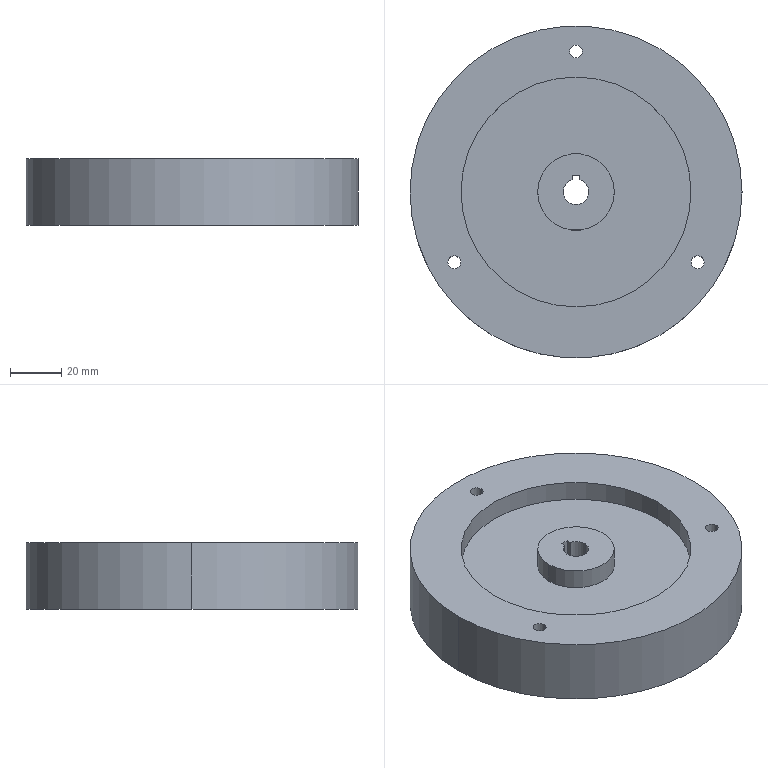Part | SolidWorks | features ICE 3, Extrusion 1 | 1 solid | 28 faces | box 130 x 130 x 26 mm | volume 250937 mm3 | cylinder 19 | plane 9 | commonest cylinder face diameters 5 x6 30 x4 90 x4 10 x3 130 x2
STEP:
#1=CARTESIAN_POINT('',(-15.,0.,8.));
#2=VERTEX_POINT('',#1);
#3=CARTESIAN_POINT('',(15.,0.,8.));
#4=VERTEX_POINT('',#3);
#5=CARTESIAN_POINT('',(0.,0.,8.));
#6=DIRECTION('',(0.,0.,-1.));
#7=DIRECTION('',(-1.,0.,0.));
#8=AXIS2_PLACEMENT_3D('',#5,#6,#7);
#9=CIRCLE('',#8,15.);
#10=EDGE_CURVE('',#2,#4,#9,.T.);
#11=ORIENTED_EDGE('',*,*,#10,.T.);
#12=CARTESIAN_POINT('',(15.,0.,0.));
#13=VERTEX_POINT('',#12);
#14=CARTESIAN_POINT('',(15.,0.,8.));
#15=DIRECTION('',(0.,0.,-1.));
#16=VECTOR('',#15,1000.);
#17=LINE('',#14,#16);
#18=EDGE_CURVE('',#4,#13,#17,.T.);
#19=ORIENTED_EDGE('',*,*,#18,.T.);
#20=CARTESIAN_POINT('',(-15.,0.,0.));
#21=VERTEX_POINT('',#20);
#22=CARTESIAN_POINT('',(0.,0.,0.));
#23=DIRECTION('',(0.,0.,-1.));
#24=DIRECTION('',(-1.,0.,0.));
#25=AXIS2_PLACEMENT_3D('',#22,#23,#24);
#26=CIRCLE('',#25,15.);
#27=EDGE_CURVE('',#21,#13,#26,.T.);
#28=ORIENTED_EDGE('',*,*,#27,.F.);
#29=CARTESIAN_POINT('',(-15.,0.,8.));
#30=DIRECTION('',(0.,0.,-1.));
#31=VECTOR('',#30,1000.);
#32=LINE('',#29,#31);
#33=EDGE_CURVE('',#2,#21,#32,.T.);
#34=ORIENTED_EDGE('',*,*,#33,.F.);
#35=EDGE_LOOP('',(#11,#19,#28,#34));
#36=FACE_OUTER_BOUND('',#35,.T.);
#37=CARTESIAN_POINT('',(0.,0.,8.));
#38=DIRECTION('',(0.,0.,-1.));
#39=DIRECTION('',(-1.,0.,0.));
#40=AXIS2_PLACEMENT_3D('',#37,#38,#39);
#41=CYLINDRICAL_SURFACE('',#40,15.);
#42=ADVANCED_FACE('',(#36),#41,.T.);
#43=CARTESIAN_POINT('',(45.,0.,8.));
#44=VERTEX_POINT('',#43);
#45=CARTESIAN_POINT('',(-45.,0.,8.));
#46=VERTEX_POINT('',#45);
#47=CARTESIAN_POINT('',(0.,0.,8.));
#48=DIRECTION('',(0.,0.,-1.));
#49=DIRECTION('',(-1.,0.,0.));
#50=AXIS2_PLACEMENT_3D('',#47,#48,#49);
#51=CIRCLE('',#50,45.);
#52=EDGE_CURVE('',#44,#46,#51,.T.);
#53=ORIENTED_EDGE('',*,*,#52,.F.);
#54=CARTESIAN_POINT('',(45.,0.,0.));
#55=VERTEX_POINT('',#54);
#56=CARTESIAN_POINT('',(45.,0.,8.));
#57=DIRECTION('',(0.,0.,-1.));
#58=VECTOR('',#57,1000.);
#59=LINE('',#56,#58);
#60=EDGE_CURVE('',#44,#55,#59,.T.);
#61=ORIENTED_EDGE('',*,*,#60,.T.);
#62=CARTESIAN_POINT('',(-45.,0.,0.));
#63=VERTEX_POINT('',#62);
#64=CARTESIAN_POINT('',(0.,0.,0.));
#65=DIRECTION('',(0.,0.,-1.));
#66=DIRECTION('',(-1.,0.,0.));
#67=AXIS2_PLACEMENT_3D('',#64,#65,#66);
#68=CIRCLE('',#67,45.);
#69=EDGE_CURVE('',#55,#63,#68,.T.);
#70=ORIENTED_EDGE('',*,*,#69,.T.);
#71=CARTESIAN_POINT('',(-45.,0.,8.));
#72=DIRECTION('',(0.,0.,-1.));
#73=VECTOR('',#72,1000.);
#74=LINE('',#71,#73);
#75=EDGE_CURVE('',#46,#63,#74,.T.);
#76=ORIENTED_EDGE('',*,*,#75,.F.);
#77=EDGE_LOOP('',(#53,#61,#70,#76));
#78=FACE_OUTER_BOUND('',#77,.T.);
#79=CARTESIAN_POINT('',(0.,0.,8.));
#80=DIRECTION('',(0.,0.,-1.));
#81=DIRECTION('',(-1.,0.,0.));
#82=AXIS2_PLACEMENT_3D('',#79,#80,#81);
#83=CYLINDRICAL_SURFACE('',#82,45.);
#84=ADVANCED_FACE('',(#78),#83,.F.);
#85=CARTESIAN_POINT('',(15.,0.,18.));
#86=VERTEX_POINT('',#85);
#87=CARTESIAN_POINT('',(-15.,0.,18.));
#88=VERTEX_POINT('',#87);
#89=CARTESIAN_POINT('',(0.,0.,18.));
#90=DIRECTION('',(0.,0.,1.));
#91=DIRECTION('',(1.,0.,0.));
#92=AXIS2_PLACEMENT_3D('',#89,#90,#91);
#93=CIRCLE('',#92,15.);
#94=EDGE_CURVE('',#86,#88,#93,.T.);
#95=ORIENTED_EDGE('',*,*,#94,.T.);
#96=CARTESIAN_POINT('',(-15.,0.,26.));
#97=VERTEX_POINT('',#96);
#98=CARTESIAN_POINT('',(-15.,0.,18.));
#99=DIRECTION('',(0.,0.,1.));
#100=VECTOR('',#99,1000.);
#101=LINE('',#98,#100);
#102=EDGE_CURVE('',#88,#97,#101,.T.);
#103=ORIENTED_EDGE('',*,*,#102,.T.);
#104=CARTESIAN_POINT('',(15.,0.,26.));
#105=VERTEX_POINT('',#104);
#106=CARTESIAN_POINT('',(0.,0.,26.));
#107=DIRECTION('',(0.,0.,1.));
#108=DIRECTION('',(1.,0.,0.));
#109=AXIS2_PLACEMENT_3D('',#106,#107,#108);
#110=CIRCLE('',#109,15.);
#111=EDGE_CURVE('',#105,#97,#110,.T.);
#112=ORIENTED_EDGE('',*,*,#111,.F.);
#113=CARTESIAN_POINT('',(15.,0.,18.));
#114=DIRECTION('',(0.,0.,1.));
#115=VECTOR('',#114,1000.);
#116=LINE('',#113,#115);
#117=EDGE_CURVE('',#86,#105,#116,.T.);
#118=ORIENTED_EDGE('',*,*,#117,.F.);
#119=EDGE_LOOP('',(#95,#103,#112,#118));
#120=FACE_OUTER_BOUND('',#119,.T.);
#121=CARTESIAN_POINT('',(0.,0.,18.));
#122=DIRECTION('',(0.,0.,1.));
#123=DIRECTION('',(1.,0.,0.));
#124=AXIS2_PLACEMENT_3D('',#121,#122,#123);
#125=CYLINDRICAL_SURFACE('',#124,15.);
#126=ADVANCED_FACE('',(#120),#125,.T.);
#127=CARTESIAN_POINT('',(-45.,0.,18.));
#128=VERTEX_POINT('',#127);
#129=CARTESIAN_POINT('',(45.,0.,18.));
#130=VERTEX_POINT('',#129);
#131=CARTESIAN_POINT('',(0.,0.,18.));
#132=DIRECTION('',(0.,0.,1.));
#133=DIRECTION('',(1.,0.,0.));
#134=AXIS2_PLACEMENT_3D('',#131,#132,#133);
#135=CIRCLE('',#134,45.);
#136=EDGE_CURVE('',#128,#130,#135,.T.);
#137=ORIENTED_EDGE('',*,*,#136,.F.);
#138=CARTESIAN_POINT('',(-45.,0.,26.));
#139=VERTEX_POINT('',#138);
#140=CARTESIAN_POINT('',(-45.,0.,18.));
#141=DIRECTION('',(0.,0.,1.));
#142=VECTOR('',#141,1000.);
#143=LINE('',#140,#142);
#144=EDGE_CURVE('',#128,#139,#143,.T.);
#145=ORIENTED_EDGE('',*,*,#144,.T.);
#146=CARTESIAN_POINT('',(45.,0.,26.));
#147=VERTEX_POINT('',#146);
#148=CARTESIAN_POINT('',(0.,0.,26.));
#149=DIRECTION('',(0.,0.,1.));
#150=DIRECTION('',(1.,0.,0.));
#151=AXIS2_PLACEMENT_3D('',#148,#149,#150);
#152=CIRCLE('',#151,45.);
#153=EDGE_CURVE('',#139,#147,#152,.T.);
#154=ORIENTED_EDGE('',*,*,#153,.T.);
#155=CARTESIAN_POINT('',(45.,0.,18.));
#156=DIRECTION('',(0.,0.,1.));
#157=VECTOR('',#156,1000.);
#158=LINE('',#155,#157);
#159=EDGE_CURVE('',#130,#147,#158,.T.);
#160=ORIENTED_EDGE('',*,*,#159,.F.);
#161=EDGE_LOOP('',(#137,#145,#154,#160));
#162=FACE_OUTER_BOUND('',#161,.T.);
#163=CARTESIAN_POINT('',(0.,0.,18.));
#164=DIRECTION('',(0.,0.,1.));
#165=DIRECTION('',(1.,0.,0.));
#166=AXIS2_PLACEMENT_3D('',#163,#164,#165);
#167=CYLINDRICAL_SURFACE('',#166,45.);
#168=ADVANCED_FACE('',(#162),#167,.F.);
#169=CARTESIAN_POINT('',(-5.,0.,0.));
#170=VERTEX_POINT('',#169);
#171=CARTESIAN_POINT('',(5.,0.,0.));
#172=VERTEX_POINT('',#171);
#173=CARTESIAN_POINT('',(0.,0.,0.));
#174=DIRECTION('',(0.,0.,1.));
#175=DIRECTION('',(1.,0.,0.));
#176=AXIS2_PLACEMENT_3D('',#173,#174,#175);
#177=CIRCLE('',#176,5.);
#178=EDGE_CURVE('',#170,#172,#177,.T.);
#179=ORIENTED_EDGE('',*,*,#178,.F.);
#180=CARTESIAN_POINT('',(-5.,0.,26.));
#181=VERTEX_POINT('',#180);
#182=CARTESIAN_POINT('',(-5.,0.,0.));
#183=DIRECTION('',(0.,0.,1.));
#184=VECTOR('',#183,1000.);
#185=LINE('',#182,#184);
#186=EDGE_CURVE('',#170,#181,#185,.T.);
#187=ORIENTED_EDGE('',*,*,#186,.T.);
#188=CARTESIAN_POINT('',(5.,0.,26.));
#189=VERTEX_POINT('',#188);
#190=CARTESIAN_POINT('',(0.,0.,26.));
#191=DIRECTION('',(0.,0.,1.));
#192=DIRECTION('',(1.,0.,0.));
#193=AXIS2_PLACEMENT_3D('',#190,#191,#192);
#194=CIRCLE('',#193,5.);
#195=EDGE_CURVE('',#181,#189,#194,.T.);
#196=ORIENTED_EDGE('',*,*,#195,.T.);
#197=CARTESIAN_POINT('',(5.,0.,0.));
#198=DIRECTION('',(0.,0.,1.));
#199=VECTOR('',#198,1000.);
#200=LINE('',#197,#199);
#201=EDGE_CURVE('',#172,#189,#200,.T.);
#202=ORIENTED_EDGE('',*,*,#201,.F.);
#203=EDGE_LOOP('',(#179,#187,#196,#202));
#204=FACE_OUTER_BOUND('',#203,.T.);
#205=CARTESIAN_POINT('',(0.,0.,0.));
#206=DIRECTION('',(0.,0.,1.));
#207=DIRECTION('',(1.,0.,0.));
#208=AXIS2_PLACEMENT_3D('',#205,#206,#207);
#209=CYLINDRICAL_SURFACE('',#208,5.);
#210=ADVANCED_FACE('',(#204),#209,.F.);
#211=CARTESIAN_POINT('',(1.5,4.77,0.));
#212=VERTEX_POINT('',#211);
#213=CARTESIAN_POINT('',(0.,0.,0.));
#214=DIRECTION('',(0.,0.,1.));
#215=DIRECTION('',(1.,0.,0.));
#216=AXIS2_PLACEMENT_3D('',#213,#214,#215);
#217=CIRCLE('',#216,5.);
#218=EDGE_CURVE('',#172,#212,#217,.T.);
#219=ORIENTED_EDGE('',*,*,#218,.F.);
#220=ORIENTED_EDGE('',*,*,#201,.T.);
#221=CARTESIAN_POINT('',(1.5,4.77,26.));
#222=VERTEX_POINT('',#221);
#223=CARTESIAN_POINT('',(0.,0.,26.));
#224=DIRECTION('',(0.,0.,1.));
#225=DIRECTION('',(1.,0.,0.));
#226=AXIS2_PLACEMENT_3D('',#223,#224,#225);
#227=CIRCLE('',#226,5.);
#228=EDGE_CURVE('',#189,#222,#227,.T.);
#229=ORIENTED_EDGE('',*,*,#228,.T.);
#230=CARTESIAN_POINT('',(1.5,4.77,0.));
#231=DIRECTION('',(0.,0.,1.));
#232=VECTOR('',#231,1000.);
#233=LINE('',#230,#232);
#234=EDGE_CURVE('',#212,#222,#233,.T.);
#235=ORIENTED_EDGE('',*,*,#234,.F.);
#236=EDGE_LOOP('',(#219,#220,#229,#235));
#237=FACE_OUTER_BOUND('',#236,.T.);
#238=CARTESIAN_POINT('',(0.,0.,0.));
#239=DIRECTION('',(0.,0.,1.));
#240=DIRECTION('',(1.,0.,0.));
#241=AXIS2_PLACEMENT_3D('',#238,#239,#240);
#242=CYLINDRICAL_SURFACE('',#241,5.);
#243=ADVANCED_FACE('',(#237),#242,.F.);
#244=CARTESIAN_POINT('',(-50.131,-27.5,26.));
#245=VERTEX_POINT('',#244);
#246=CARTESIAN_POINT('',(-45.131,-27.5,26.));
#247=VERTEX_POINT('',#246);
#248=CARTESIAN_POINT('',(-47.631,-27.5,26.));
#249=DIRECTION('',(0.,0.,1.));
#250=DIRECTION('',(1.,0.,0.));
#251=AXIS2_PLACEMENT_3D('',#248,#249,#250);
#252=CIRCLE('',#251,2.5);
#253=EDGE_CURVE('',#245,#247,#252,.T.);
#254=ORIENTED_EDGE('',*,*,#253,.T.);
#255=CARTESIAN_POINT('',(-45.131,-27.5,0.));
#256=VERTEX_POINT('',#255);
#257=CARTESIAN_POINT('',(-45.131,-27.5,26.));
#258=DIRECTION('',(0.,0.,-1.));
#259=VECTOR('',#258,1000.);
#260=LINE('',#257,#259);
#261=EDGE_CURVE('',#247,#256,#260,.T.);
#262=ORIENTED_EDGE('',*,*,#261,.T.);
#263=CARTESIAN_POINT('',(-50.131,-27.5,0.));
#264=VERTEX_POINT('',#263);
#265=CARTESIAN_POINT('',(-47.631,-27.5,0.));
#266=DIRECTION('',(0.,0.,1.));
#267=DIRECTION('',(1.,0.,0.));
#268=AXIS2_PLACEMENT_3D('',#265,#266,#267);
#269=CIRCLE('',#268,2.5);
#270=EDGE_CURVE('',#264,#256,#269,.T.);
#271=ORIENTED_EDGE('',*,*,#270,.F.);
#272=CARTESIAN_POINT('',(-50.131,-27.5,26.));
#273=DIRECTION('',(0.,0.,-1.));
#274=VECTOR('',#273,1000.);
#275=LINE('',#272,#274);
#276=EDGE_CURVE('',#245,#264,#275,.T.);
#277=ORIENTED_EDGE('',*,*,#276,.F.);
#278=EDGE_LOOP('',(#254,#262,#271,#277));
#279=FACE_OUTER_BOUND('',#278,.T.);
#280=CARTESIAN_POINT('',(-47.631,-27.5,26.));
#281=DIRECTION('',(0.,0.,-1.));
#282=DIRECTION('',(-1.,0.,0.));
#283=AXIS2_PLACEMENT_3D('',#280,#281,#282);
#284=CYLINDRICAL_SURFACE('',#283,2.5);
#285=ADVANCED_FACE('',(#279),#284,.F.);
#286=CARTESIAN_POINT('',(45.131,-27.5,26.));
#287=VERTEX_POINT('',#286);
#288=CARTESIAN_POINT('',(50.131,-27.5,26.));
#289=VERTEX_POINT('',#288);
#290=CARTESIAN_POINT('',(47.631,-27.5,26.));
#291=DIRECTION('',(0.,0.,1.));
#292=DIRECTION('',(1.,0.,0.));
#293=AXIS2_PLACEMENT_3D('',#290,#291,#292);
#294=CIRCLE('',#293,2.5);
#295=EDGE_CURVE('',#287,#289,#294,.T.);
#296=ORIENTED_EDGE('',*,*,#295,.T.);
#297=CARTESIAN_POINT('',(50.131,-27.5,0.));
#298=VERTEX_POINT('',#297);
#299=CARTESIAN_POINT('',(50.131,-27.5,26.));
#300=DIRECTION('',(0.,0.,-1.));
#301=VECTOR('',#300,1000.);
#302=LINE('',#299,#301);
#303=EDGE_CURVE('',#289,#298,#302,.T.);
#304=ORIENTED_EDGE('',*,*,#303,.T.);
#305=CARTESIAN_POINT('',(45.131,-27.5,0.));
#306=VERTEX_POINT('',#305);
#307=CARTESIAN_POINT('',(47.631,-27.5,0.));
#308=DIRECTION('',(0.,0.,1.));
#309=DIRECTION('',(1.,0.,0.));
#310=AXIS2_PLACEMENT_3D('',#307,#308,#309);
#311=CIRCLE('',#310,2.5);
#312=EDGE_CURVE('',#306,#298,#311,.T.);
#313=ORIENTED_EDGE('',*,*,#312,.F.);
#314=CARTESIAN_POINT('',(45.131,-27.5,26.));
#315=DIRECTION('',(0.,0.,-1.));
#316=VECTOR('',#315,1000.);
#317=LINE('',#314,#316);
#318=EDGE_CURVE('',#287,#306,#317,.T.);
#319=ORIENTED_EDGE('',*,*,#318,.F.);
#320=EDGE_LOOP('',(#296,#304,#313,#319));
#321=FACE_OUTER_BOUND('',#320,.T.);
#322=CARTESIAN_POINT('',(47.631,-27.5,26.));
#323=DIRECTION('',(0.,0.,-1.));
#324=DIRECTION('',(-1.,0.,0.));
#325=AXIS2_PLACEMENT_3D('',#322,#323,#324);
#326=CYLINDRICAL_SURFACE('',#325,2.5);
#327=ADVANCED_FACE('',(#321),#326,.F.);
#328=CARTESIAN_POINT('',(-2.5,55.,26.));
#329=VERTEX_POINT('',#328);
#330=CARTESIAN_POINT('',(2.5,55.,26.));
#331=VERTEX_POINT('',#330);
#332=CARTESIAN_POINT('',(0.,55.,26.));
#333=DIRECTION('',(0.,0.,1.));
#334=DIRECTION('',(1.,0.,0.));
#335=AXIS2_PLACEMENT_3D('',#332,#333,#334);
#336=CIRCLE('',#335,2.5);
#337=EDGE_CURVE('',#329,#331,#336,.T.);
#338=ORIENTED_EDGE('',*,*,#337,.T.);
#339=CARTESIAN_POINT('',(2.5,55.,0.));
#340=VERTEX_POINT('',#339);
#341=CARTESIAN_POINT('',(2.5,55.,26.));
#342=DIRECTION('',(0.,0.,-1.));
#343=VECTOR('',#342,1000.);
#344=LINE('',#341,#343);
#345=EDGE_CURVE('',#331,#340,#344,.T.);
#346=ORIENTED_EDGE('',*,*,#345,.T.);
#347=CARTESIAN_POINT('',(-2.5,55.,0.));
#348=VERTEX_POINT('',#347);
#349=CARTESIAN_POINT('',(0.,55.,0.));
#350=DIRECTION('',(0.,0.,1.));
#351=DIRECTION('',(1.,0.,0.));
#352=AXIS2_PLACEMENT_3D('',#349,#350,#351);
#353=CIRCLE('',#352,2.5);
#354=EDGE_CURVE('',#348,#340,#353,.T.);
#355=ORIENTED_EDGE('',*,*,#354,.F.);
#356=CARTESIAN_POINT('',(-2.5,55.,26.));
#357=DIRECTION('',(0.,0.,-1.));
#358=VECTOR('',#357,1000.);
#359=LINE('',#356,#358);
#360=EDGE_CURVE('',#329,#348,#359,.T.);
#361=ORIENTED_EDGE('',*,*,#360,.F.);
#362=EDGE_LOOP('',(#338,#346,#355,#361));
#363=FACE_OUTER_BOUND('',#362,.T.);
#364=CARTESIAN_POINT('',(0.,55.,26.));
#365=DIRECTION('',(0.,0.,-1.));
#366=DIRECTION('',(-1.,0.,0.));
#367=AXIS2_PLACEMENT_3D('',#364,#365,#366);
#368=CYLINDRICAL_SURFACE('',#367,2.5);
#369=ADVANCED_FACE('',(#363),#368,.F.);
#370=CARTESIAN_POINT('',(65.,0.,26.));
#371=VERTEX_POINT('',#370);
#372=CARTESIAN_POINT('',(-65.,0.,26.));
#373=VERTEX_POINT('',#372);
#374=CARTESIAN_POINT('',(0.,0.,26.));
#375=DIRECTION('',(0.,0.,1.));
#376=DIRECTION('',(1.,0.,0.));
#377=AXIS2_PLACEMENT_3D('',#374,#375,#376);
#378=CIRCLE('',#377,65.);
#379=EDGE_CURVE('',#371,#373,#378,.T.);
#380=ORIENTED_EDGE('',*,*,#379,.F.);
#381=CARTESIAN_POINT('',(65.,0.,0.));
#382=VERTEX_POINT('',#381);
#383=CARTESIAN_POINT('',(65.,0.,26.));
#384=DIRECTION('',(0.,0.,-1.));
#385=VECTOR('',#384,1000.);
#386=LINE('',#383,#385);
#387=EDGE_CURVE('',#371,#382,#386,.T.);
#388=ORIENTED_EDGE('',*,*,#387,.T.);
#389=CARTESIAN_POINT('',(-65.,0.,0.));
#390=VERTEX_POINT('',#389);
#391=CARTESIAN_POINT('',(0.,0.,0.));
#392=DIRECTION('',(0.,0.,1.));
#393=DIRECTION('',(1.,0.,0.));
#394=AXIS2_PLACEMENT_3D('',#391,#392,#393);
#395=CIRCLE('',#394,65.);
#396=EDGE_CURVE('',#382,#390,#395,.T.);
#397=ORIENTED_EDGE('',*,*,#396,.T.);
#398=CARTESIAN_POINT('',(-65.,0.,26.));
#399=DIRECTION('',(0.,0.,-1.));
#400=VECTOR('',#399,1000.);
#401=LINE('',#398,#400);
#402=EDGE_CURVE('',#373,#390,#401,.T.);
#403=ORIENTED_EDGE('',*,*,#402,.F.);
#404=EDGE_LOOP('',(#380,#388,#397,#403));
#405=FACE_OUTER_BOUND('',#404,.T.);
#406=CARTESIAN_POINT('',(0.,0.,26.));
#407=DIRECTION('',(0.,0.,-1.));
#408=DIRECTION('',(-1.,0.,0.));
#409=AXIS2_PLACEMENT_3D('',#406,#407,#408);
#410=CYLINDRICAL_SURFACE('',#409,65.);
#411=ADVANCED_FACE('',(#405),#410,.T.);
#412=CARTESIAN_POINT('',(1.5,6.403,0.));
#413=VERTEX_POINT('',#412);
#414=CARTESIAN_POINT('',(-1.5,6.403,0.));
#415=VERTEX_POINT('',#414);
#416=CARTESIAN_POINT('',(-1.5,6.403,0.));
#417=DIRECTION('',(-1.,0.,0.));
#418=VECTOR('',#417,1000.);
#419=LINE('',#416,#418);
#420=EDGE_CURVE('',#413,#415,#419,.T.);
#421=ORIENTED_EDGE('',*,*,#420,.T.);
#422=CARTESIAN_POINT('',(-1.5,4.77,0.));
#423=VERTEX_POINT('',#422);
#424=CARTESIAN_POINT('',(-1.5,6.403,0.));
#425=DIRECTION('',(0.,-1.,0.));
#426=VECTOR('',#425,1000.);
#427=LINE('',#424,#426);
#428=EDGE_CURVE('',#415,#423,#427,.T.);
#429=ORIENTED_EDGE('',*,*,#428,.T.);
#430=CARTESIAN_POINT('',(0.,0.,0.));
#431=DIRECTION('',(0.,0.,1.));
#432=DIRECTION('',(1.,0.,0.));
#433=AXIS2_PLACEMENT_3D('',#430,#431,#432);
#434=CIRCLE('',#433,5.);
#435=EDGE_CURVE('',#423,#170,#434,.T.);
#436=ORIENTED_EDGE('',*,*,#435,.T.);
#437=ORIENTED_EDGE('',*,*,#178,.T.);
#438=ORIENTED_EDGE('',*,*,#218,.T.);
#439=CARTESIAN_POINT('',(1.5,6.403,0.));
#440=DIRECTION('',(0.,1.,0.));
#441=VECTOR('',#440,1000.);
#442=LINE('',#439,#441);
#443=EDGE_CURVE('',#212,#413,#442,.T.);
#444=ORIENTED_EDGE('',*,*,#443,.T.);
#445=EDGE_LOOP('',(#421,#429,#436,#437,#438,#444));
#446=FACE_BOUND('',#445,.T.);
#447=ORIENTED_EDGE('',*,*,#27,.T.);
#448=CARTESIAN_POINT('',(0.,0.,0.));
#449=DIRECTION('',(0.,0.,-1.));
#450=DIRECTION('',(-1.,0.,0.));
#451=AXIS2_PLACEMENT_3D('',#448,#449,#450);
#452=CIRCLE('',#451,15.);
#453=EDGE_CURVE('',#13,#21,#452,.T.);
#454=ORIENTED_EDGE('',*,*,#453,.T.);
#455=EDGE_LOOP('',(#447,#454));
#456=FACE_OUTER_BOUND('',#455,.T.);
#457=CARTESIAN_POINT('',(0.,0.,0.));
#458=DIRECTION('',(0.,0.,1.));
#459=DIRECTION('',(1.,0.,0.));
#460=AXIS2_PLACEMENT_3D('',#457,#458,#459);
#461=PLANE('',#460);
#462=ADVANCED_FACE('',(#446,#456),#461,.F.);
#463=CARTESIAN_POINT('',(-1.5,6.403,26.));
#464=VERTEX_POINT('',#463);
#465=CARTESIAN_POINT('',(-1.5,4.77,26.));
#466=VERTEX_POINT('',#465);
#467=CARTESIAN_POINT('',(-1.5,6.403,26.));
#468=DIRECTION('',(0.,-1.,0.));
#469=VECTOR('',#468,1000.);
#470=LINE('',#467,#469);
#471=EDGE_CURVE('',#464,#466,#470,.T.);
#472=ORIENTED_EDGE('',*,*,#471,.F.);
#473=CARTESIAN_POINT('',(1.5,6.403,26.));
#474=VERTEX_POINT('',#473);
#475=CARTESIAN_POINT('',(-1.5,6.403,26.));
#476=DIRECTION('',(-1.,0.,0.));
#477=VECTOR('',#476,1000.);
#478=LINE('',#475,#477);
#479=EDGE_CURVE('',#474,#464,#478,.T.);
#480=ORIENTED_EDGE('',*,*,#479,.F.);
#481=CARTESIAN_POINT('',(1.5,6.403,26.));
#482=DIRECTION('',(0.,1.,0.));
#483=VECTOR('',#482,1000.);
#484=LINE('',#481,#483);
#485=EDGE_CURVE('',#222,#474,#484,.T.);
#486=ORIENTED_EDGE('',*,*,#485,.F.);
#487=ORIENTED_EDGE('',*,*,#228,.F.);
#488=ORIENTED_EDGE('',*,*,#195,.F.);
#489=CARTESIAN_POINT('',(0.,0.,26.));
#490=DIRECTION('',(0.,0.,1.));
#491=DIRECTION('',(1.,0.,0.));
#492=AXIS2_PLACEMENT_3D('',#489,#490,#491);
#493=CIRCLE('',#492,5.);
#494=EDGE_CURVE('',#466,#181,#493,.T.);
#495=ORIENTED_EDGE('',*,*,#494,.F.);
#496=EDGE_LOOP('',(#472,#480,#486,#487,#488,#495));
#497=FACE_BOUND('',#496,.T.);
#498=ORIENTED_EDGE('',*,*,#111,.T.);
#499=CARTESIAN_POINT('',(0.,0.,26.));
#500=DIRECTION('',(0.,0.,1.));
#501=DIRECTION('',(1.,0.,0.));
#502=AXIS2_PLACEMENT_3D('',#499,#500,#501);
#503=CIRCLE('',#502,15.);
#504=EDGE_CURVE('',#97,#105,#503,.T.);
#505=ORIENTED_EDGE('',*,*,#504,.T.);
#506=EDGE_LOOP('',(#498,#505));
#507=FACE_OUTER_BOUND('',#506,.T.);
#508=CARTESIAN_POINT('',(0.,0.,26.));
#509=DIRECTION('',(0.,0.,1.));
#510=DIRECTION('',(1.,0.,0.));
#511=AXIS2_PLACEMENT_3D('',#508,#509,#510);
#512=PLANE('',#511);
#513=ADVANCED_FACE('',(#497,#507),#512,.T.);
#514=CARTESIAN_POINT('',(0.,0.,26.));
#515=DIRECTION('',(0.,0.,1.));
#516=DIRECTION('',(1.,0.,0.));
#517=AXIS2_PLACEMENT_3D('',#514,#515,#516);
#518=CIRCLE('',#517,45.);
#519=EDGE_CURVE('',#147,#139,#518,.T.);
#520=ORIENTED_EDGE('',*,*,#519,.F.);
#521=ORIENTED_EDGE('',*,*,#153,.F.);
#522=EDGE_LOOP('',(#520,#521));
#523=FACE_BOUND('',#522,.T.);
#524=ORIENTED_EDGE('',*,*,#295,.F.);
#525=CARTESIAN_POINT('',(47.631,-27.5,26.));
#526=DIRECTION('',(0.,0.,1.));
#527=DIRECTION('',(1.,0.,0.));
#528=AXIS2_PLACEMENT_3D('',#525,#526,#527);
#529=CIRCLE('',#528,2.5);
#530=EDGE_CURVE('',#289,#287,#529,.T.);
#531=ORIENTED_EDGE('',*,*,#530,.F.);
#532=EDGE_LOOP('',(#524,#531));
#533=FACE_BOUND('',#532,.T.);
#534=CARTESIAN_POINT('',(0.,0.,26.));
#535=DIRECTION('',(0.,0.,1.));
#536=DIRECTION('',(1.,0.,0.));
#537=AXIS2_PLACEMENT_3D('',#534,#535,#536);
#538=CIRCLE('',#537,65.);
#539=EDGE_CURVE('',#373,#371,#538,.T.);
#540=ORIENTED_EDGE('',*,*,#539,.T.);
#541=ORIENTED_EDGE('',*,*,#379,.T.);
#542=EDGE_LOOP('',(#540,#541));
#543=FACE_OUTER_BOUND('',#542,.T.);
#544=ORIENTED_EDGE('',*,*,#337,.F.);
#545=CARTESIAN_POINT('',(0.,55.,26.));
#546=DIRECTION('',(0.,0.,1.));
#547=DIRECTION('',(1.,0.,0.));
#548=AXIS2_PLACEMENT_3D('',#545,#546,#547);
#549=CIRCLE('',#548,2.5);
#550=EDGE_CURVE('',#331,#329,#549,.T.);
#551=ORIENTED_EDGE('',*,*,#550,.F.);
#552=EDGE_LOOP('',(#544,#551));
#553=FACE_BOUND('',#552,.T.);
#554=ORIENTED_EDGE('',*,*,#253,.F.);
#555=CARTESIAN_POINT('',(-47.631,-27.5,26.));
#556=DIRECTION('',(0.,0.,1.));
#557=DIRECTION('',(1.,0.,0.));
#558=AXIS2_PLACEMENT_3D('',#555,#556,#557);
#559=CIRCLE('',#558,2.5);
#560=EDGE_CURVE('',#247,#245,#559,.T.);
#561=ORIENTED_EDGE('',*,*,#560,.F.);
#562=EDGE_LOOP('',(#554,#561));
#563=FACE_BOUND('',#562,.T.);
#564=CARTESIAN_POINT('',(0.,0.,26.));
#565=DIRECTION('',(0.,0.,1.));
#566=DIRECTION('',(1.,0.,0.));
#567=AXIS2_PLACEMENT_3D('',#564,#565,#566);
#568=PLANE('',#567);
#569=ADVANCED_FACE('',(#523,#533,#543,#553,#563),#568,.T.);
#570=CARTESIAN_POINT('',(0.,0.,0.));
#571=DIRECTION('',(0.,0.,-1.));
#572=DIRECTION('',(-1.,0.,0.));
#573=AXIS2_PLACEMENT_3D('',#570,#571,#572);
#574=CIRCLE('',#573,45.);
#575=EDGE_CURVE('',#63,#55,#574,.T.);
#576=ORIENTED_EDGE('',*,*,#575,.F.);
#577=ORIENTED_EDGE('',*,*,#69,.F.);
#578=EDGE_LOOP('',(#576,#577));
#579=FACE_BOUND('',#578,.T.);
#580=CARTESIAN_POINT('',(0.,0.,0.));
#581=DIRECTION('',(0.,0.,1.));
#582=DIRECTION('',(1.,0.,0.));
#583=AXIS2_PLACEMENT_3D('',#580,#581,#582);
#584=CIRCLE('',#583,65.);
#585=EDGE_CURVE('',#390,#382,#584,.T.);
#586=ORIENTED_EDGE('',*,*,#585,.F.);
#587=ORIENTED_EDGE('',*,*,#396,.F.);
#588=EDGE_LOOP('',(#586,#587));
#589=FACE_OUTER_BOUND('',#588,.T.);
#590=ORIENTED_EDGE('',*,*,#354,.T.);
#591=CARTESIAN_POINT('',(0.,55.,0.));
#592=DIRECTION('',(0.,0.,1.));
#593=DIRECTION('',(1.,0.,0.));
#594=AXIS2_PLACEMENT_3D('',#591,#592,#593);
#595=CIRCLE('',#594,2.5);
#596=EDGE_CURVE('',#340,#348,#595,.T.);
#597=ORIENTED_EDGE('',*,*,#596,.T.);
#598=EDGE_LOOP('',(#590,#597));
#599=FACE_BOUND('',#598,.T.);
#600=ORIENTED_EDGE('',*,*,#312,.T.);
#601=CARTESIAN_POINT('',(47.631,-27.5,0.));
#602=DIRECTION('',(0.,0.,1.));
#603=DIRECTION('',(1.,0.,0.));
#604=AXIS2_PLACEMENT_3D('',#601,#602,#603);
#605=CIRCLE('',#604,2.5);
#606=EDGE_CURVE('',#298,#306,#605,.T.);
#607=ORIENTED_EDGE('',*,*,#606,.T.);
#608=EDGE_LOOP('',(#600,#607));
#609=FACE_BOUND('',#608,.T.);
#610=ORIENTED_EDGE('',*,*,#270,.T.);
#611=CARTESIAN_POINT('',(-47.631,-27.5,0.));
#612=DIRECTION('',(0.,0.,1.));
#613=DIRECTION('',(1.,0.,0.));
#614=AXIS2_PLACEMENT_3D('',#611,#612,#613);
#615=CIRCLE('',#614,2.5);
#616=EDGE_CURVE('',#256,#264,#615,.T.);
#617=ORIENTED_EDGE('',*,*,#616,.T.);
#618=EDGE_LOOP('',(#610,#617));
#619=FACE_BOUND('',#618,.T.);
#620=CARTESIAN_POINT('',(0.,0.,0.));
#621=DIRECTION('',(0.,0.,1.));
#622=DIRECTION('',(1.,0.,0.));
#623=AXIS2_PLACEMENT_3D('',#620,#621,#622);
#624=PLANE('',#623);
#625=ADVANCED_FACE('',(#579,#589,#599,#609,#619),#624,.F.);
#626=ORIENTED_EDGE('',*,*,#387,.F.);
#627=ORIENTED_EDGE('',*,*,#539,.F.);
#628=ORIENTED_EDGE('',*,*,#402,.T.);
#629=ORIENTED_EDGE('',*,*,#585,.T.);
#630=EDGE_LOOP('',(#626,#627,#628,#629));
#631=FACE_OUTER_BOUND('',#630,.T.);
#632=CARTESIAN_POINT('',(0.,0.,26.));
#633=DIRECTION('',(0.,0.,-1.));
#634=DIRECTION('',(-1.,0.,0.));
#635=AXIS2_PLACEMENT_3D('',#632,#633,#634);
#636=CYLINDRICAL_SURFACE('',#635,65.);
#637=ADVANCED_FACE('',(#631),#636,.T.);
#638=ORIENTED_EDGE('',*,*,#345,.F.);
#639=ORIENTED_EDGE('',*,*,#550,.T.);
#640=ORIENTED_EDGE('',*,*,#360,.T.);
#641=ORIENTED_EDGE('',*,*,#596,.F.);
#642=EDGE_LOOP('',(#638,#639,#640,#641));
#643=FACE_OUTER_BOUND('',#642,.T.);
#644=CARTESIAN_POINT('',(0.,55.,26.));
#645=DIRECTION('',(0.,0.,-1.));
#646=DIRECTION('',(-1.,0.,0.));
#647=AXIS2_PLACEMENT_3D('',#644,#645,#646);
#648=CYLINDRICAL_SURFACE('',#647,2.5);
#649=ADVANCED_FACE('',(#643),#648,.F.);
#650=ORIENTED_EDGE('',*,*,#303,.F.);
#651=ORIENTED_EDGE('',*,*,#530,.T.);
#652=ORIENTED_EDGE('',*,*,#318,.T.);
#653=ORIENTED_EDGE('',*,*,#606,.F.);
#654=EDGE_LOOP('',(#650,#651,#652,#653));
#655=FACE_OUTER_BOUND('',#654,.T.);
#656=CARTESIAN_POINT('',(47.631,-27.5,26.));
#657=DIRECTION('',(0.,0.,-1.));
#658=DIRECTION('',(-1.,0.,0.));
#659=AXIS2_PLACEMENT_3D('',#656,#657,#658);
#660=CYLINDRICAL_SURFACE('',#659,2.5);
#661=ADVANCED_FACE('',(#655),#660,.F.);
#662=ORIENTED_EDGE('',*,*,#261,.F.);
#663=ORIENTED_EDGE('',*,*,#560,.T.);
#664=ORIENTED_EDGE('',*,*,#276,.T.);
#665=ORIENTED_EDGE('',*,*,#616,.F.);
#666=EDGE_LOOP('',(#662,#663,#664,#665));
#667=FACE_OUTER_BOUND('',#666,.T.);
#668=CARTESIAN_POINT('',(-47.631,-27.5,26.));
#669=DIRECTION('',(0.,0.,-1.));
#670=DIRECTION('',(-1.,0.,0.));
#671=AXIS2_PLACEMENT_3D('',#668,#669,#670);
#672=CYLINDRICAL_SURFACE('',#671,2.5);
#673=ADVANCED_FACE('',(#667),#672,.F.);
#674=ORIENTED_EDGE('',*,*,#471,.T.);
#675=CARTESIAN_POINT('',(-1.5,4.77,0.));
#676=DIRECTION('',(0.,0.,1.));
#677=VECTOR('',#676,1000.);
#678=LINE('',#675,#677);
#679=EDGE_CURVE('',#423,#466,#678,.T.);
#680=ORIENTED_EDGE('',*,*,#679,.F.);
#681=ORIENTED_EDGE('',*,*,#428,.F.);
#682=CARTESIAN_POINT('',(-1.5,6.403,0.));
#683=DIRECTION('',(0.,0.,1.));
#684=VECTOR('',#683,1000.);
#685=LINE('',#682,#684);
#686=EDGE_CURVE('',#415,#464,#685,.T.);
#687=ORIENTED_EDGE('',*,*,#686,.T.);
#688=EDGE_LOOP('',(#674,#680,#681,#687));
#689=FACE_OUTER_BOUND('',#688,.T.);
#690=CARTESIAN_POINT('',(-1.5,6.403,0.));
#691=DIRECTION('',(-1.,0.,0.));
#692=DIRECTION('',(0.,-1.,0.));
#693=AXIS2_PLACEMENT_3D('',#690,#691,#692);
#694=PLANE('',#693);
#695=ADVANCED_FACE('',(#689),#694,.F.);
#696=ORIENTED_EDGE('',*,*,#479,.T.);
#697=ORIENTED_EDGE('',*,*,#686,.F.);
#698=ORIENTED_EDGE('',*,*,#420,.F.);
#699=CARTESIAN_POINT('',(1.5,6.403,0.));
#700=DIRECTION('',(0.,0.,1.));
#701=VECTOR('',#700,1000.);
#702=LINE('',#699,#701);
#703=EDGE_CURVE('',#413,#474,#702,.T.);
#704=ORIENTED_EDGE('',*,*,#703,.T.);
#705=EDGE_LOOP('',(#696,#697,#698,#704));
#706=FACE_OUTER_BOUND('',#705,.T.);
#707=CARTESIAN_POINT('',(-1.5,6.403,0.));
#708=DIRECTION('',(0.,1.,0.));
#709=DIRECTION('',(0.,0.,1.));
#710=AXIS2_PLACEMENT_3D('',#707,#708,#709);
#711=PLANE('',#710);
#712=ADVANCED_FACE('',(#706),#711,.F.);
#713=ORIENTED_EDGE('',*,*,#485,.T.);
#714=ORIENTED_EDGE('',*,*,#703,.F.);
#715=ORIENTED_EDGE('',*,*,#443,.F.);
#716=ORIENTED_EDGE('',*,*,#234,.T.);
#717=EDGE_LOOP('',(#713,#714,#715,#716));
#718=FACE_OUTER_BOUND('',#717,.T.);
#719=CARTESIAN_POINT('',(1.5,6.403,0.));
#720=DIRECTION('',(1.,0.,0.));
#721=DIRECTION('',(0.,1.,0.));
#722=AXIS2_PLACEMENT_3D('',#719,#720,#721);
#723=PLANE('',#722);
#724=ADVANCED_FACE('',(#718),#723,.F.);
#725=ORIENTED_EDGE('',*,*,#186,.F.);
#726=ORIENTED_EDGE('',*,*,#435,.F.);
#727=ORIENTED_EDGE('',*,*,#679,.T.);
#728=ORIENTED_EDGE('',*,*,#494,.T.);
#729=EDGE_LOOP('',(#725,#726,#727,#728));
#730=FACE_OUTER_BOUND('',#729,.T.);
#731=CARTESIAN_POINT('',(0.,0.,0.));
#732=DIRECTION('',(0.,0.,1.));
#733=DIRECTION('',(1.,0.,0.));
#734=AXIS2_PLACEMENT_3D('',#731,#732,#733);
#735=CYLINDRICAL_SURFACE('',#734,5.);
#736=ADVANCED_FACE('',(#730),#735,.F.);
#737=ORIENTED_EDGE('',*,*,#144,.F.);
#738=CARTESIAN_POINT('',(0.,0.,18.));
#739=DIRECTION('',(0.,0.,1.));
#740=DIRECTION('',(1.,0.,0.));
#741=AXIS2_PLACEMENT_3D('',#738,#739,#740);
#742=CIRCLE('',#741,45.);
#743=EDGE_CURVE('',#130,#128,#742,.T.);
#744=ORIENTED_EDGE('',*,*,#743,.F.);
#745=ORIENTED_EDGE('',*,*,#159,.T.);
#746=ORIENTED_EDGE('',*,*,#519,.T.);
#747=EDGE_LOOP('',(#737,#744,#745,#746));
#748=FACE_OUTER_BOUND('',#747,.T.);
#749=CARTESIAN_POINT('',(0.,0.,18.));
#750=DIRECTION('',(0.,0.,1.));
#751=DIRECTION('',(1.,0.,0.));
#752=AXIS2_PLACEMENT_3D('',#749,#750,#751);
#753=CYLINDRICAL_SURFACE('',#752,45.);
#754=ADVANCED_FACE('',(#748),#753,.F.);
#755=ORIENTED_EDGE('',*,*,#94,.F.);
#756=CARTESIAN_POINT('',(0.,0.,18.));
#757=DIRECTION('',(0.,0.,1.));
#758=DIRECTION('',(1.,0.,0.));
#759=AXIS2_PLACEMENT_3D('',#756,#757,#758);
#760=CIRCLE('',#759,15.);
#761=EDGE_CURVE('',#88,#86,#760,.T.);
#762=ORIENTED_EDGE('',*,*,#761,.F.);
#763=EDGE_LOOP('',(#755,#762));
#764=FACE_BOUND('',#763,.T.);
#765=ORIENTED_EDGE('',*,*,#743,.T.);
#766=ORIENTED_EDGE('',*,*,#136,.T.);
#767=EDGE_LOOP('',(#765,#766));
#768=FACE_OUTER_BOUND('',#767,.T.);
#769=CARTESIAN_POINT('',(0.,0.,18.));
#770=DIRECTION('',(0.,0.,1.));
#771=DIRECTION('',(1.,0.,0.));
#772=AXIS2_PLACEMENT_3D('',#769,#770,#771);
#773=PLANE('',#772);
#774=ADVANCED_FACE('',(#764,#768),#773,.T.);
#775=ORIENTED_EDGE('',*,*,#102,.F.);
#776=ORIENTED_EDGE('',*,*,#761,.T.);
#777=ORIENTED_EDGE('',*,*,#117,.T.);
#778=ORIENTED_EDGE('',*,*,#504,.F.);
#779=EDGE_LOOP('',(#775,#776,#777,#778));
#780=FACE_OUTER_BOUND('',#779,.T.);
#781=CARTESIAN_POINT('',(0.,0.,18.));
#782=DIRECTION('',(0.,0.,1.));
#783=DIRECTION('',(1.,0.,0.));
#784=AXIS2_PLACEMENT_3D('',#781,#782,#783);
#785=CYLINDRICAL_SURFACE('',#784,15.);
#786=ADVANCED_FACE('',(#780),#785,.T.);
#787=ORIENTED_EDGE('',*,*,#60,.F.);
#788=CARTESIAN_POINT('',(0.,0.,8.));
#789=DIRECTION('',(0.,0.,-1.));
#790=DIRECTION('',(-1.,0.,0.));
#791=AXIS2_PLACEMENT_3D('',#788,#789,#790);
#792=CIRCLE('',#791,45.);
#793=EDGE_CURVE('',#46,#44,#792,.T.);
#794=ORIENTED_EDGE('',*,*,#793,.F.);
#795=ORIENTED_EDGE('',*,*,#75,.T.);
#796=ORIENTED_EDGE('',*,*,#575,.T.);
#797=EDGE_LOOP('',(#787,#794,#795,#796));
#798=FACE_OUTER_BOUND('',#797,.T.);
#799=CARTESIAN_POINT('',(0.,0.,8.));
#800=DIRECTION('',(0.,0.,-1.));
#801=DIRECTION('',(-1.,0.,0.));
#802=AXIS2_PLACEMENT_3D('',#799,#800,#801);
#803=CYLINDRICAL_SURFACE('',#802,45.);
#804=ADVANCED_FACE('',(#798),#803,.F.);
#805=ORIENTED_EDGE('',*,*,#10,.F.);
#806=CARTESIAN_POINT('',(0.,0.,8.));
#807=DIRECTION('',(0.,0.,-1.));
#808=DIRECTION('',(-1.,0.,0.));
#809=AXIS2_PLACEMENT_3D('',#806,#807,#808);
#810=CIRCLE('',#809,15.);
#811=EDGE_CURVE('',#4,#2,#810,.T.);
#812=ORIENTED_EDGE('',*,*,#811,.F.);
#813=EDGE_LOOP('',(#805,#812));
#814=FACE_BOUND('',#813,.T.);
#815=ORIENTED_EDGE('',*,*,#793,.T.);
#816=ORIENTED_EDGE('',*,*,#52,.T.);
#817=EDGE_LOOP('',(#815,#816));
#818=FACE_OUTER_BOUND('',#817,.T.);
#819=CARTESIAN_POINT('',(0.,0.,8.));
#820=DIRECTION('',(0.,0.,-1.));
#821=DIRECTION('',(-1.,0.,0.));
#822=AXIS2_PLACEMENT_3D('',#819,#820,#821);
#823=PLANE('',#822);
#824=ADVANCED_FACE('',(#814,#818),#823,.T.);
#825=ORIENTED_EDGE('',*,*,#18,.F.);
#826=ORIENTED_EDGE('',*,*,#811,.T.);
#827=ORIENTED_EDGE('',*,*,#33,.T.);
#828=ORIENTED_EDGE('',*,*,#453,.F.);
#829=EDGE_LOOP('',(#825,#826,#827,#828));
#830=FACE_OUTER_BOUND('',#829,.T.);
#831=CARTESIAN_POINT('',(0.,0.,8.));
#832=DIRECTION('',(0.,0.,-1.));
#833=DIRECTION('',(-1.,0.,0.));
#834=AXIS2_PLACEMENT_3D('',#831,#832,#833);
#835=CYLINDRICAL_SURFACE('',#834,15.);
#836=ADVANCED_FACE('',(#830),#835,.T.);
#837=CLOSED_SHELL('',(#42,#84,#126,#168,#210,#243,#285,#327,#369,#411,#462,#513,#569,#625,#637,#649,#661,#673,#695,#712,#724,#736,#754,#774,#786,#804,#824,#836));
#838=MANIFOLD_SOLID_BREP('',#837);
#839=CARTESIAN_POINT('',(0.,0.,0.));
#840=DIRECTION('',(0.,0.,1.));
#841=DIRECTION('',(1.,0.,0.));
#842=AXIS2_PLACEMENT_3D('',#839,#840,#841);
#843=(LENGTH_UNIT()NAMED_UNIT(*)SI_UNIT(.MILLI.,.METRE.));
#844=UNCERTAINTY_MEASURE_WITH_UNIT(LENGTH_MEASURE(0.00001),#843,'','');
#845=(NAMED_UNIT(*)PLANE_ANGLE_UNIT()SI_UNIT($,.RADIAN.));
#846=(NAMED_UNIT(*)SI_UNIT($,.STERADIAN.)SOLID_ANGLE_UNIT());
#847=(GEOMETRIC_REPRESENTATION_CONTEXT(3)GLOBAL_UNCERTAINTY_ASSIGNED_CONTEXT((#844))GLOBAL_UNIT_ASSIGNED_CONTEXT((#843,#845,#846))REPRESENTATION_CONTEXT('',''));
#848=ADVANCED_BREP_SHAPE_REPRESENTATION('',(#838,#842),#847);